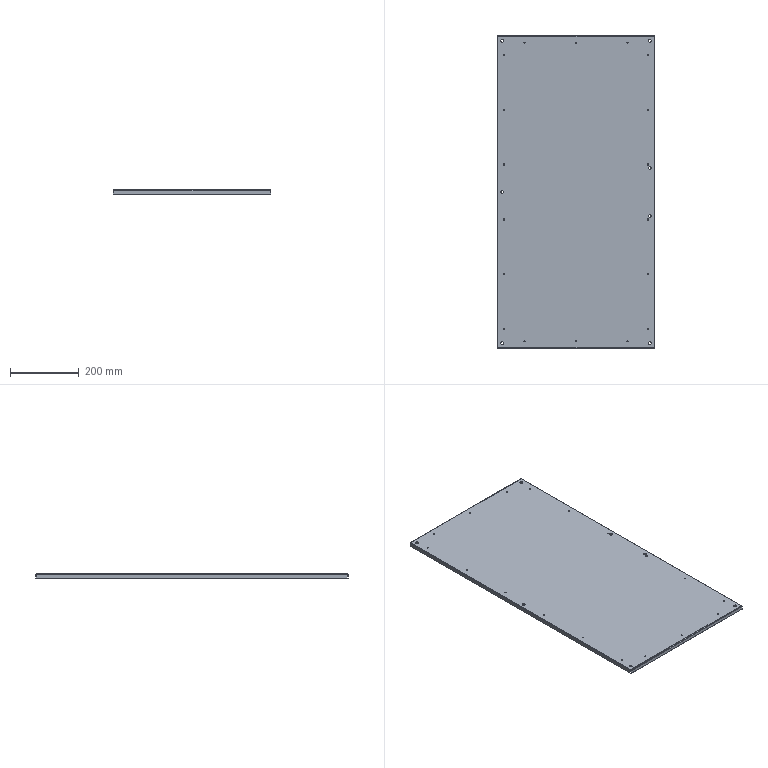Part | SolidWorks | features EdgeFlange 4, 3DProfileFeature 3, HoleWzd 3, MirrorPattern 3, FlatPattern 1, SMBaseFlange 1, SheetMetal 1 | 1 solid | 92 faces | box 460 x 910 x 12 mm | volume 667248 mm3 | cylinder 58 | plane 34 | commonest cylinder face diameters 3.3 x36 8 x14 2 x3 5 x3 0.2 x1 3.2 x1